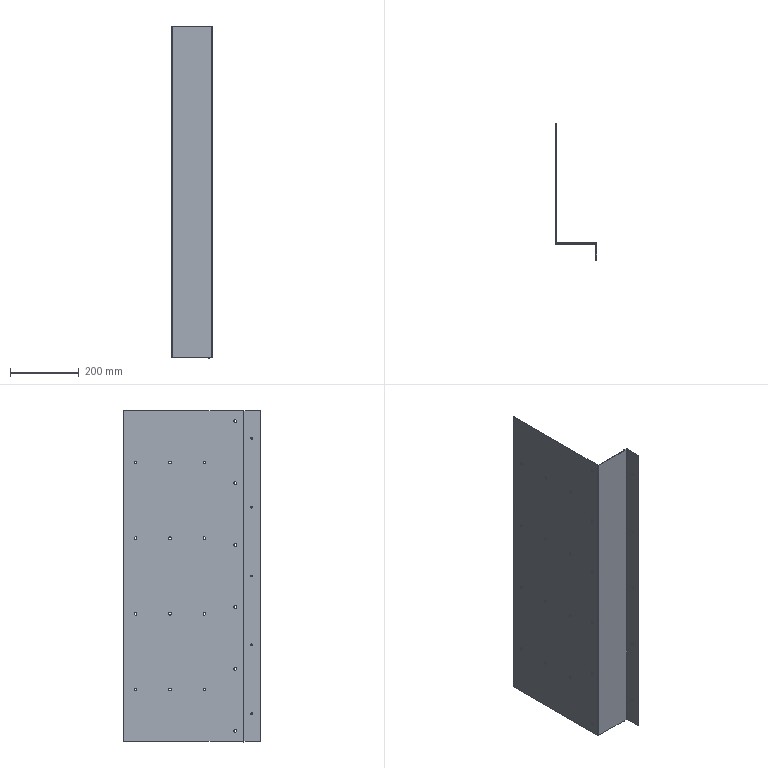Part | STEP file | SX-006-03 | 1 solid | 76 faces | box 120 x 398 x 965.5 mm | volume 988273 mm3 | cylinder 50 | plane 26 | commonest cylinder face diameters 8 x36 5.4 x10 0.4 x2 4.4 x2